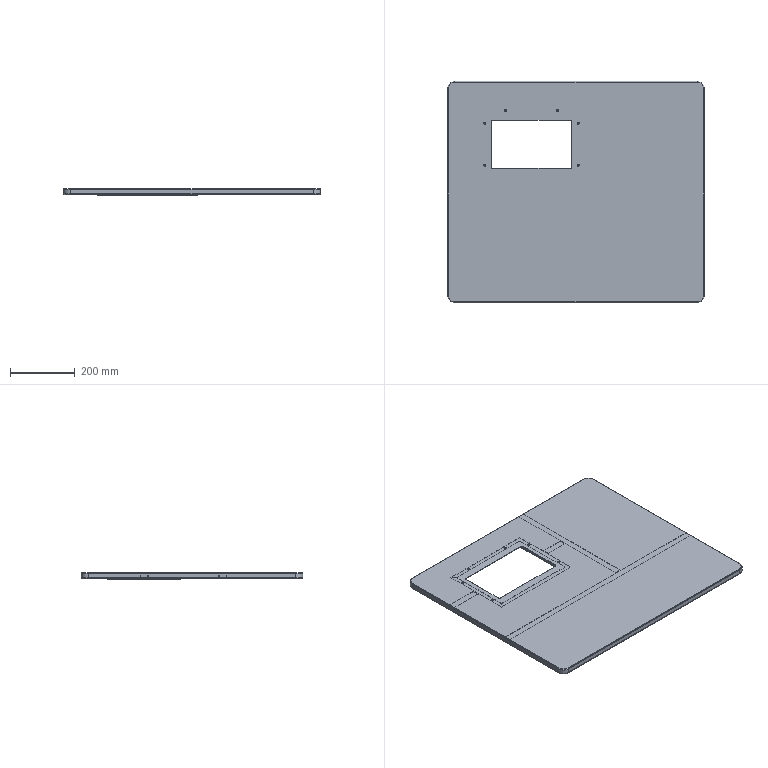Part | STEP file | Front door panel lower V1.201001_default<by machining> | 9 solids | 406 faces | box 796 x 686 x 21.5 mm | volume 1058682 mm3 | plane 210 | cylinder 180 | torus 16 | commonest cylinder face diameters 3.5 x32 6.5 x32 2.5 x24 3 x16 5 x16 6 x16